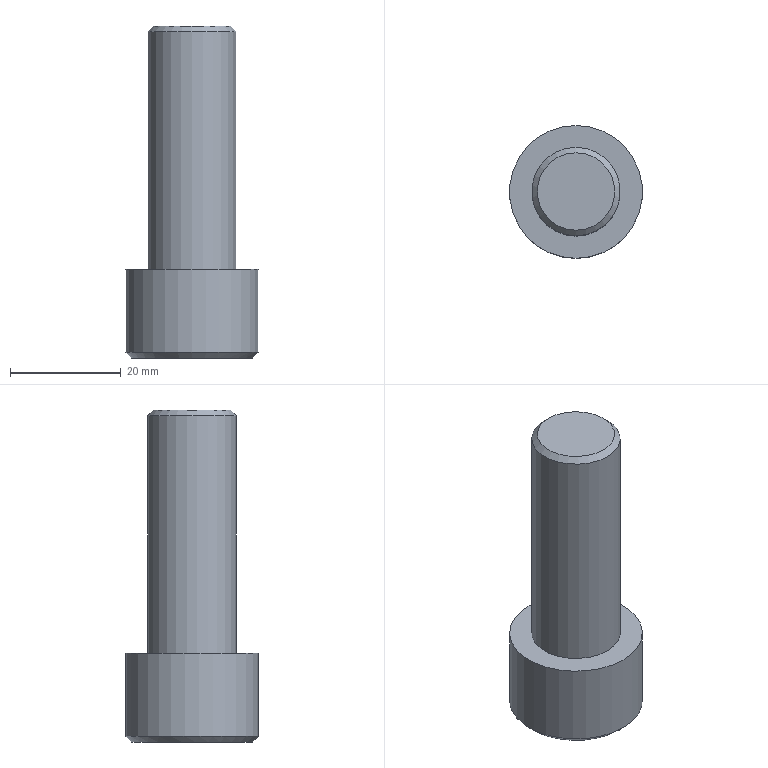Part | STEP file | solid 207 | 1 solid | 14 faces | box 24 x 24 x 60 mm | volume 14836 mm3 | plane 10 | cone 2 | cylinder 2 | commonest cylinder face diameters 16 x1 24 x1